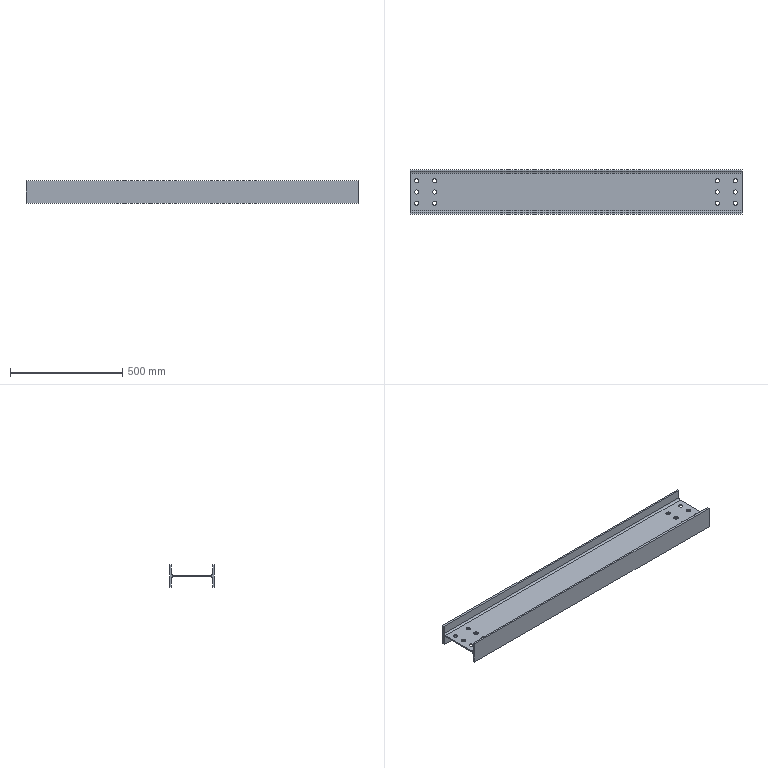Part | STEP file | 电柜通道主梁1主体_Default<As Machined> | 1 solid | 42 faces | box 1480 x 200 x 100 mm | volume 3928355 mm3 | cylinder 28 | plane 14 | commonest cylinder face diameters 19 x24 16 x4